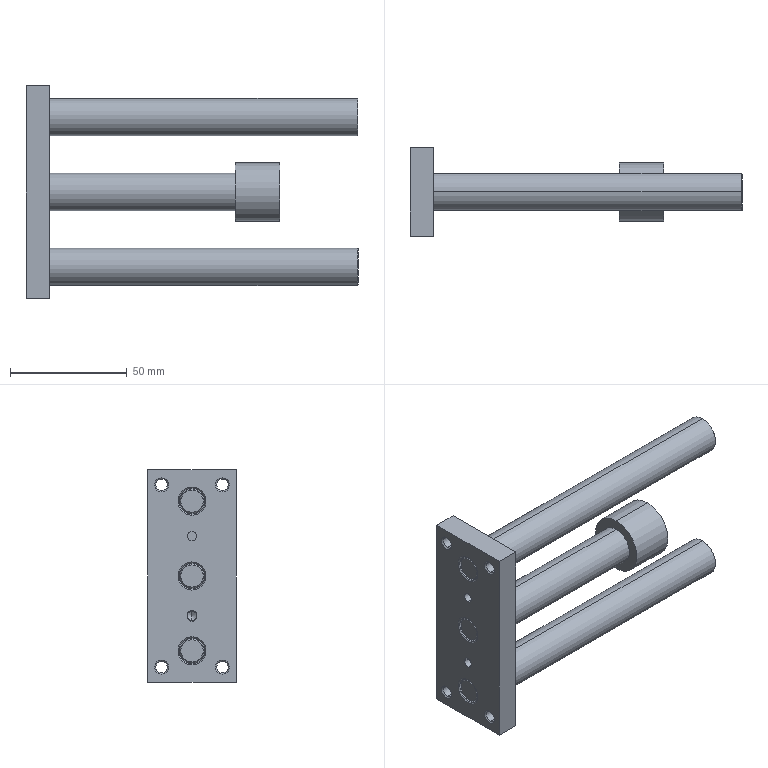Part | SolidWorks | features BaseBody 1 | 1 solid | 90 faces | box 142 x 38 x 91 mm | volume 111727 mm3 | cylinder 35 | cone 34 | plane 21 | commonest cylinder face diameters 4.917 x8 4 x7 10.5 x6 11 x6 16 x6 25 x2